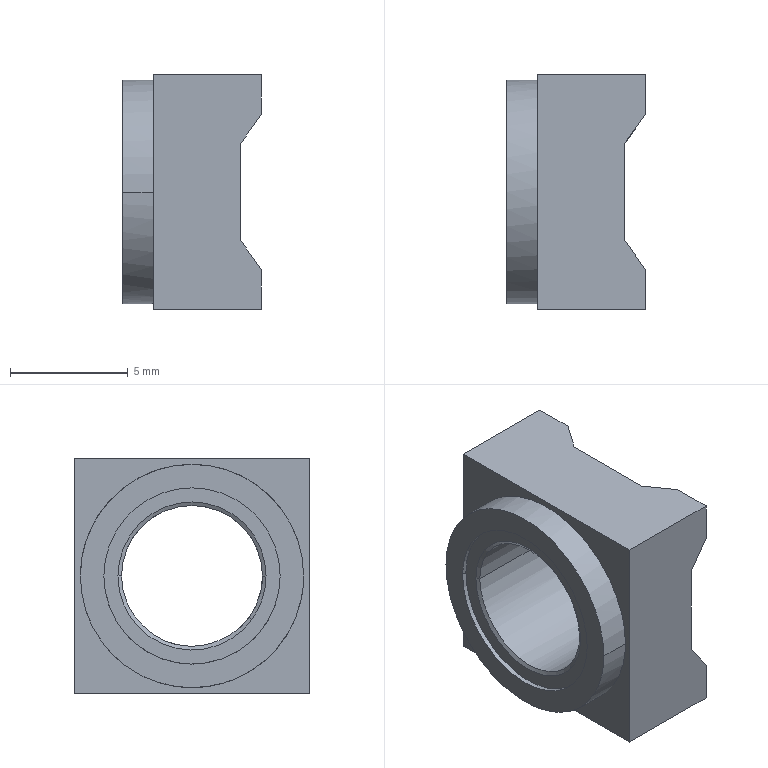Part | NX | features BREP 1 | 1 solid | 28 faces | box 5.9 x 10 x 10 mm | volume 326.565 mm3 | plane 16 | cylinder 6 | cone 6 | commonest cylinder face diameters 6 x2 7.5 x2 9.5 x2